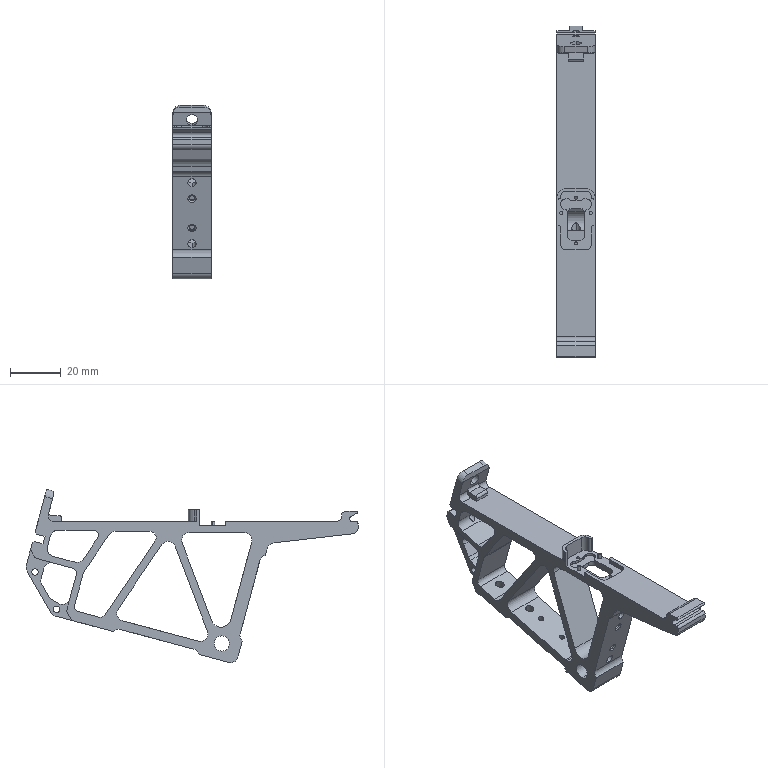Part | SolidWorks | features BaseBody 1 | 1 solid | 205 faces | box 15 x 130.973 x 68.389 mm | volume 25082 mm3 | cylinder 112 | plane 85 | cone 8 | commonest cylinder face diameters 6 x30 4 x29 1.25 x8 2 x8 2.2 x8 2.5 x8